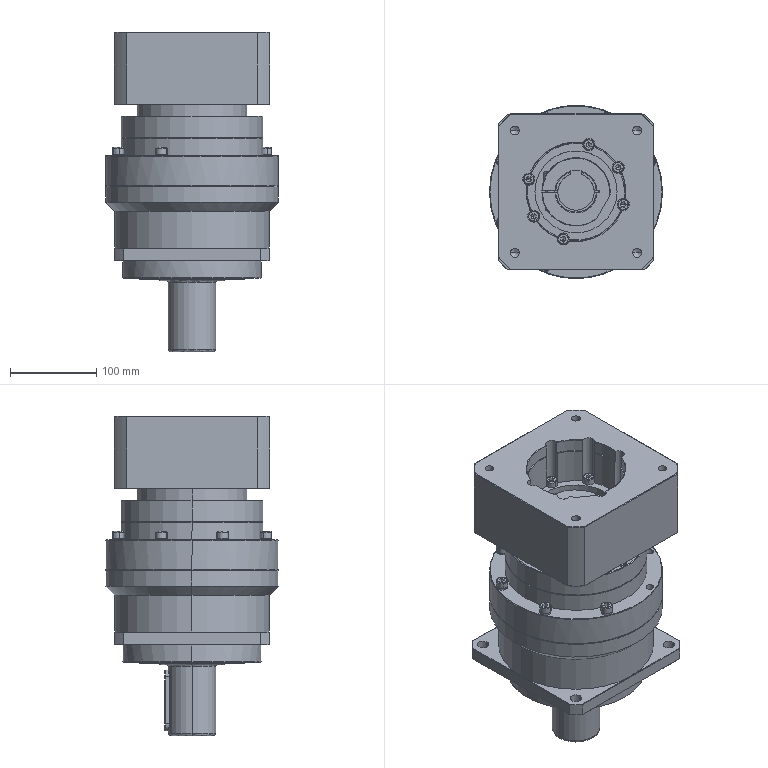Part | SolidWorks | 44 solids | 1156 faces | box 200 x 200 x 369.495 mm | volume 7118058 mm3 | plane 506 | cylinder 422 | cone 184 | spline 44 | commonest cylinder face diameters 8.68 x54 12.88 x54 4 x40 9 x40 8 x36 13 x36